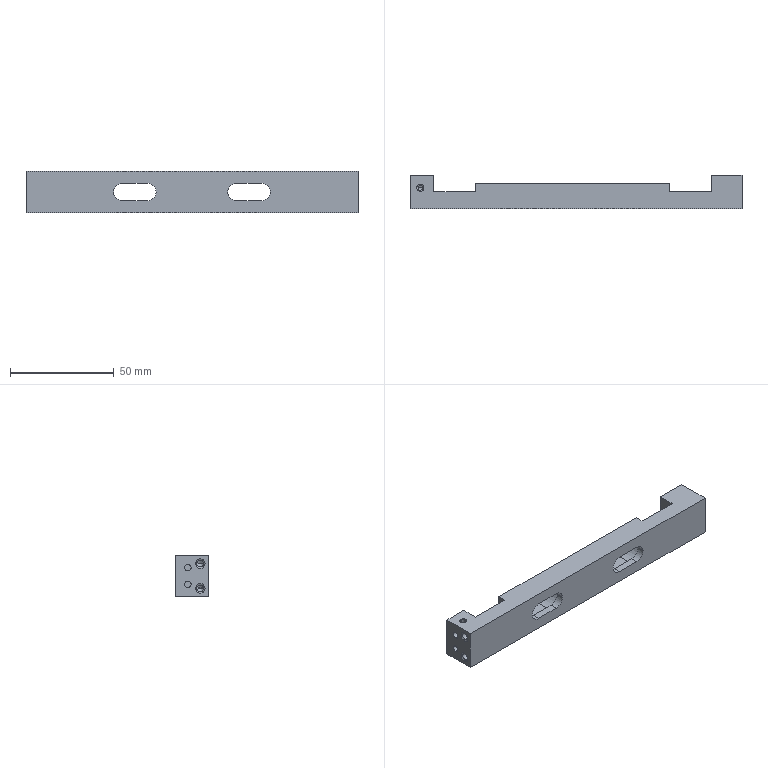Part | NX | 1 solid | 60 faces | box 160 x 16 x 20 mm | volume 29927 mm3 | plane 24 | cylinder 24 | cone 12 | commonest cylinder face diameters 8.5 x6 14.5 x6 2.5 x4 3.1 x4 3.3 x4